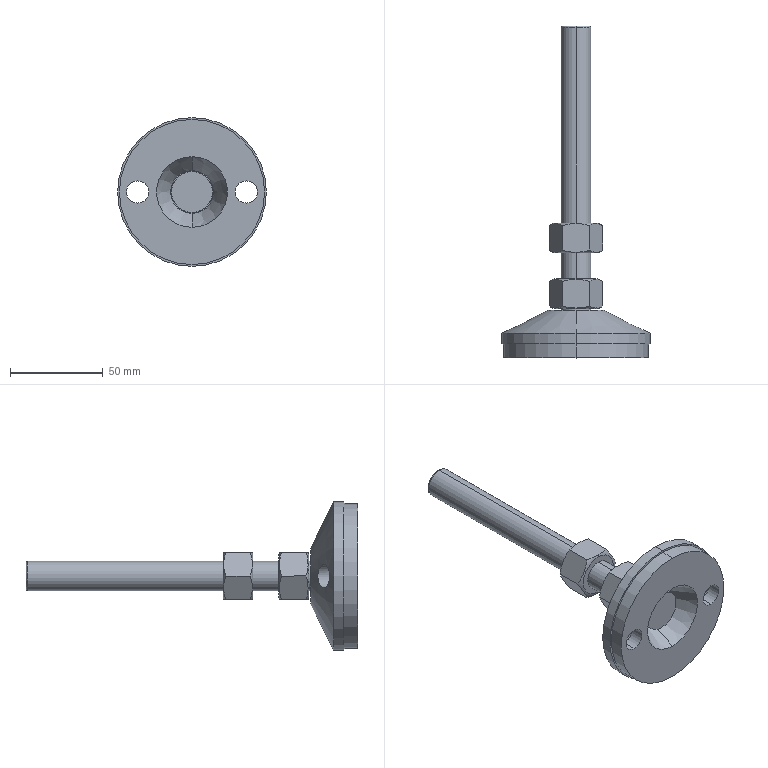Part | SolidWorks | features HoleWzd 2, Revolution 2, Fillet 1, ICE 1, LPattern 1, RevCut 1 | 2 solids | 68 faces | box 80 x 178.5 x 80 mm | volume 123669 mm3 | plane 26 | cylinder 24 | torus 10 | cone 8 | commonest cylinder face diameters 16 x10 12 x4 12.5 x4 22 x2 78 x2 80 x2